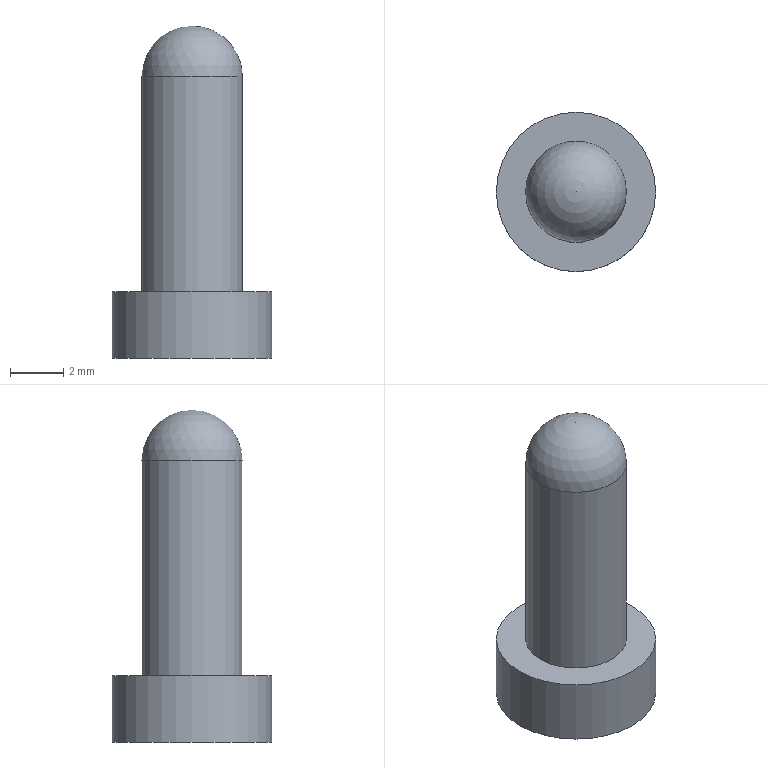Part | NX | features solid 2 | 1 solid | 5 faces | box 6 x 6 x 12.5 mm | volume 176.915 mm3 | cylinder 2 | plane 2 | sphere 1 | commonest cylinder face diameters 3.8 x1 6 x1
STEP:
#1=CARTESIAN_POINT('',(282.1,-130.972,-52.9));
#2=VERTEX_POINT('',#1);
#3=CARTESIAN_POINT('',(284.,-130.972,-52.9));
#4=DIRECTION('',(0.,0.,1.));
#5=DIRECTION('',(-1.,0.,0.));
#6=AXIS2_PLACEMENT_3D('',#3,#4,#5);
#7=CIRCLE('',#6,1.9);
#8=EDGE_CURVE('',#2,#2,#7,.T.);
#9=ORIENTED_EDGE('',*,*,#8,.F.);
#10=EDGE_LOOP('',(#9));
#11=FACE_BOUND('',#10,.T.);
#12=CARTESIAN_POINT('',(282.1,-130.972,-61.));
#13=VERTEX_POINT('',#12);
#14=CARTESIAN_POINT('',(284.,-130.972,-61.));
#15=DIRECTION('',(0.,0.,1.));
#16=DIRECTION('',(-1.,0.,0.));
#17=AXIS2_PLACEMENT_3D('',#14,#15,#16);
#18=CIRCLE('',#17,1.9);
#19=EDGE_CURVE('',#13,#13,#18,.T.);
#20=ORIENTED_EDGE('',*,*,#19,.T.);
#21=EDGE_LOOP('',(#20));
#22=FACE_BOUND('',#21,.T.);
#23=CARTESIAN_POINT('',(284.,-130.972,-61.));
#24=DIRECTION('',(0.,0.,1.));
#25=DIRECTION('',(1.,0.,0.));
#26=AXIS2_PLACEMENT_3D('',#23,#24,#25);
#27=CYLINDRICAL_SURFACE('',#26,1.9);
#28=ADVANCED_FACE('',(#11,#22),#27,.T.);
#29=ORIENTED_EDGE('',*,*,#8,.T.);
#30=EDGE_LOOP('',(#29));
#31=FACE_BOUND('',#30,.T.);
#32=CARTESIAN_POINT('',(284.,-130.972,-52.9));
#33=DIRECTION('',(0.,0.,1.));
#34=DIRECTION('',(1.,0.,0.));
#35=AXIS2_PLACEMENT_3D('',#32,#33,#34);
#36=SPHERICAL_SURFACE('',#35,1.9);
#37=ADVANCED_FACE('',(#31),#36,.T.);
#38=CARTESIAN_POINT('',(281.,-130.972,-63.5));
#39=VERTEX_POINT('',#38);
#40=CARTESIAN_POINT('',(284.,-130.972,-63.5));
#41=DIRECTION('',(0.,0.,-1.));
#42=DIRECTION('',(-1.,0.,0.));
#43=AXIS2_PLACEMENT_3D('',#40,#41,#42);
#44=CIRCLE('',#43,3.);
#45=EDGE_CURVE('',#39,#39,#44,.T.);
#46=ORIENTED_EDGE('',*,*,#45,.F.);
#47=EDGE_LOOP('',(#46));
#48=FACE_BOUND('',#47,.T.);
#49=CARTESIAN_POINT('',(281.,-130.972,-61.));
#50=VERTEX_POINT('',#49);
#51=CARTESIAN_POINT('',(284.,-130.972,-61.));
#52=DIRECTION('',(0.,0.,-1.));
#53=DIRECTION('',(-1.,0.,0.));
#54=AXIS2_PLACEMENT_3D('',#51,#52,#53);
#55=CIRCLE('',#54,3.);
#56=EDGE_CURVE('',#50,#50,#55,.T.);
#57=ORIENTED_EDGE('',*,*,#56,.T.);
#58=EDGE_LOOP('',(#57));
#59=FACE_BOUND('',#58,.T.);
#60=CARTESIAN_POINT('',(284.,-130.972,-63.5));
#61=DIRECTION('',(0.,0.,1.));
#62=DIRECTION('',(1.,0.,0.));
#63=AXIS2_PLACEMENT_3D('',#60,#61,#62);
#64=CYLINDRICAL_SURFACE('',#63,3.);
#65=ADVANCED_FACE('',(#48,#59),#64,.T.);
#66=ORIENTED_EDGE('',*,*,#45,.T.);
#67=EDGE_LOOP('',(#66));
#68=FACE_BOUND('',#67,.T.);
#69=CARTESIAN_POINT('',(284.,-130.972,-63.5));
#70=DIRECTION('',(0.,0.,1.));
#71=DIRECTION('',(1.,0.,0.));
#72=AXIS2_PLACEMENT_3D('',#69,#70,#71);
#73=PLANE('',#72);
#74=ADVANCED_FACE('',(#68),#73,.F.);
#75=ORIENTED_EDGE('',*,*,#19,.F.);
#76=EDGE_LOOP('',(#75));
#77=FACE_BOUND('',#76,.T.);
#78=ORIENTED_EDGE('',*,*,#56,.F.);
#79=EDGE_LOOP('',(#78));
#80=FACE_BOUND('',#79,.T.);
#81=CARTESIAN_POINT('',(284.,-130.972,-61.));
#82=DIRECTION('',(0.,0.,1.));
#83=DIRECTION('',(1.,0.,0.));
#84=AXIS2_PLACEMENT_3D('',#81,#82,#83);
#85=PLANE('',#84);
#86=ADVANCED_FACE('',(#77,#80),#85,.T.);
#87=CLOSED_SHELL('',(#28,#37,#65,#74,#86));
#88=MANIFOLD_SOLID_BREP('',#87);
#89=(LENGTH_UNIT()NAMED_UNIT(*)SI_UNIT(.MILLI.,.METRE.));
#90=UNCERTAINTY_MEASURE_WITH_UNIT(LENGTH_MEASURE(0.00001),#89,'','');
#91=(NAMED_UNIT(*)PLANE_ANGLE_UNIT()SI_UNIT($,.RADIAN.));
#92=(NAMED_UNIT(*)SI_UNIT($,.STERADIAN.)SOLID_ANGLE_UNIT());
#93=(GEOMETRIC_REPRESENTATION_CONTEXT(3)GLOBAL_UNCERTAINTY_ASSIGNED_CONTEXT((#90))GLOBAL_UNIT_ASSIGNED_CONTEXT((#89,#91,#92))REPRESENTATION_CONTEXT('',''));
#94=ADVANCED_BREP_SHAPE_REPRESENTATION('',(#88),#93);